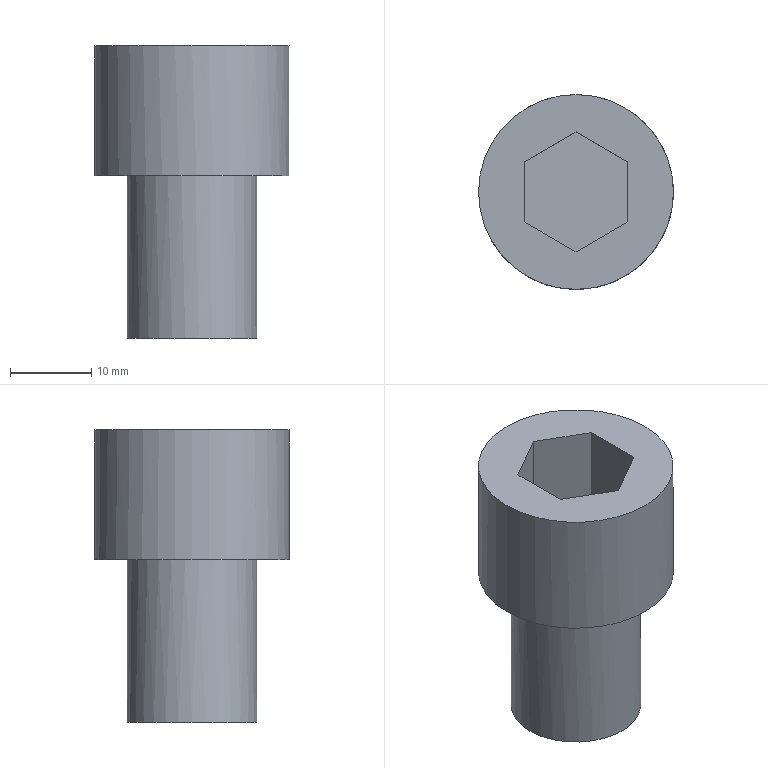Part | NX | features solid 2 | 1 solid | 12 faces | box 24 x 24 x 36 mm | volume 9897 mm3 | plane 10 | cylinder 2 | commonest cylinder face diameters 16 x1 24 x1
STEP:
#1=CARTESIAN_POINT('',(1036.4,273.695,-259.));
#2=VERTEX_POINT('',#1);
#3=CARTESIAN_POINT('',(1030.,277.39,-259.));
#4=VERTEX_POINT('',#3);
#5=CARTESIAN_POINT('',(1033.2,275.543,-259.));
#6=DIRECTION('',(-0.866,0.5,0.));
#7=VECTOR('',#6,1000.);
#8=LINE('',#5,#7);
#9=EDGE_CURVE('',#2,#4,#8,.T.);
#10=ORIENTED_EDGE('',*,*,#9,.F.);
#11=CARTESIAN_POINT('',(1036.4,266.305,-259.));
#12=VERTEX_POINT('',#11);
#13=CARTESIAN_POINT('',(1036.4,270.,-259.));
#14=DIRECTION('',(0.,1.,0.));
#15=VECTOR('',#14,1000.);
#16=LINE('',#13,#15);
#17=EDGE_CURVE('',#12,#2,#16,.T.);
#18=ORIENTED_EDGE('',*,*,#17,.F.);
#19=CARTESIAN_POINT('',(1030.,262.61,-259.));
#20=VERTEX_POINT('',#19);
#21=CARTESIAN_POINT('',(1033.2,264.457,-259.));
#22=DIRECTION('',(0.866,0.5,0.));
#23=VECTOR('',#22,1000.);
#24=LINE('',#21,#23);
#25=EDGE_CURVE('',#20,#12,#24,.T.);
#26=ORIENTED_EDGE('',*,*,#25,.F.);
#27=CARTESIAN_POINT('',(1023.6,266.305,-259.));
#28=VERTEX_POINT('',#27);
#29=CARTESIAN_POINT('',(1026.8,264.457,-259.));
#30=DIRECTION('',(0.866,-0.5,0.));
#31=VECTOR('',#30,1000.);
#32=LINE('',#29,#31);
#33=EDGE_CURVE('',#28,#20,#32,.T.);
#34=ORIENTED_EDGE('',*,*,#33,.F.);
#35=CARTESIAN_POINT('',(1023.6,273.695,-259.));
#36=VERTEX_POINT('',#35);
#37=CARTESIAN_POINT('',(1023.6,270.,-259.));
#38=DIRECTION('',(0.,-1.,0.));
#39=VECTOR('',#38,1000.);
#40=LINE('',#37,#39);
#41=EDGE_CURVE('',#36,#28,#40,.T.);
#42=ORIENTED_EDGE('',*,*,#41,.F.);
#43=CARTESIAN_POINT('',(1026.8,275.543,-259.));
#44=DIRECTION('',(-0.866,-0.5,0.));
#45=VECTOR('',#44,1000.);
#46=LINE('',#43,#45);
#47=EDGE_CURVE('',#4,#36,#46,.T.);
#48=ORIENTED_EDGE('',*,*,#47,.F.);
#49=EDGE_LOOP('',(#10,#18,#26,#34,#42,#48));
#50=FACE_BOUND('',#49,.T.);
#51=CARTESIAN_POINT('',(1042.,270.,-259.));
#52=VERTEX_POINT('',#51);
#53=CARTESIAN_POINT('',(1030.,270.,-259.));
#54=DIRECTION('',(0.,0.,-1.));
#55=DIRECTION('',(1.,0.,0.));
#56=AXIS2_PLACEMENT_3D('',#53,#54,#55);
#57=CIRCLE('',#56,12.);
#58=EDGE_CURVE('',#52,#52,#57,.T.);
#59=ORIENTED_EDGE('',*,*,#58,.F.);
#60=EDGE_LOOP('',(#59));
#61=FACE_BOUND('',#60,.T.);
#62=CARTESIAN_POINT('',(1030.,270.,-259.));
#63=DIRECTION('',(0.,0.,1.));
#64=DIRECTION('',(-1.,0.,0.));
#65=AXIS2_PLACEMENT_3D('',#62,#63,#64);
#66=PLANE('',#65);
#67=ADVANCED_FACE('',(#50,#61),#66,.T.);
#68=CARTESIAN_POINT('',(1038.,270.,-275.));
#69=VERTEX_POINT('',#68);
#70=CARTESIAN_POINT('',(1030.,270.,-275.));
#71=DIRECTION('',(0.,0.,-1.));
#72=DIRECTION('',(1.,0.,0.));
#73=AXIS2_PLACEMENT_3D('',#70,#71,#72);
#74=CIRCLE('',#73,8.);
#75=EDGE_CURVE('',#69,#69,#74,.T.);
#76=ORIENTED_EDGE('',*,*,#75,.F.);
#77=EDGE_LOOP('',(#76));
#78=FACE_BOUND('',#77,.T.);
#79=CARTESIAN_POINT('',(1018.,270.,-275.));
#80=VERTEX_POINT('',#79);
#81=CARTESIAN_POINT('',(1030.,270.,-275.));
#82=DIRECTION('',(0.,0.,1.));
#83=DIRECTION('',(-1.,0.,0.));
#84=AXIS2_PLACEMENT_3D('',#81,#82,#83);
#85=CIRCLE('',#84,12.);
#86=EDGE_CURVE('',#80,#80,#85,.T.);
#87=ORIENTED_EDGE('',*,*,#86,.F.);
#88=EDGE_LOOP('',(#87));
#89=FACE_BOUND('',#88,.T.);
#90=CARTESIAN_POINT('',(1030.,270.,-275.));
#91=DIRECTION('',(0.,0.,-1.));
#92=DIRECTION('',(1.,0.,0.));
#93=AXIS2_PLACEMENT_3D('',#90,#91,#92);
#94=PLANE('',#93);
#95=ADVANCED_FACE('',(#78,#89),#94,.T.);
#96=ORIENTED_EDGE('',*,*,#58,.T.);
#97=EDGE_LOOP('',(#96));
#98=FACE_BOUND('',#97,.T.);
#99=ORIENTED_EDGE('',*,*,#86,.T.);
#100=EDGE_LOOP('',(#99));
#101=FACE_BOUND('',#100,.T.);
#102=CARTESIAN_POINT('',(1030.,270.,-275.));
#103=DIRECTION('',(0.,0.,1.));
#104=DIRECTION('',(-1.,0.,0.));
#105=AXIS2_PLACEMENT_3D('',#102,#103,#104);
#106=CYLINDRICAL_SURFACE('',#105,12.);
#107=ADVANCED_FACE('',(#98,#101),#106,.T.);
#108=ORIENTED_EDGE('',*,*,#9,.T.);
#109=CARTESIAN_POINT('',(1030.,277.39,-268.6));
#110=VERTEX_POINT('',#109);
#111=CARTESIAN_POINT('',(1030.,277.39,-268.6));
#112=DIRECTION('',(0.,0.,1.));
#113=VECTOR('',#112,1000.);
#114=LINE('',#111,#113);
#115=EDGE_CURVE('',#110,#4,#114,.T.);
#116=ORIENTED_EDGE('',*,*,#115,.F.);
#117=CARTESIAN_POINT('',(1036.4,273.695,-268.6));
#118=VERTEX_POINT('',#117);
#119=CARTESIAN_POINT('',(1036.4,273.695,-268.6));
#120=DIRECTION('',(-0.866,0.5,0.));
#121=VECTOR('',#120,1000.);
#122=LINE('',#119,#121);
#123=EDGE_CURVE('',#118,#110,#122,.T.);
#124=ORIENTED_EDGE('',*,*,#123,.F.);
#125=CARTESIAN_POINT('',(1036.4,273.695,-268.6));
#126=DIRECTION('',(0.,0.,1.));
#127=VECTOR('',#126,1000.);
#128=LINE('',#125,#127);
#129=EDGE_CURVE('',#118,#2,#128,.T.);
#130=ORIENTED_EDGE('',*,*,#129,.T.);
#131=EDGE_LOOP('',(#108,#116,#124,#130));
#132=FACE_BOUND('',#131,.T.);
#133=CARTESIAN_POINT('',(1033.2,275.543,-260.6));
#134=DIRECTION('',(0.5,0.866,0.));
#135=DIRECTION('',(-0.866,0.5,0.));
#136=AXIS2_PLACEMENT_3D('',#133,#134,#135);
#137=PLANE('',#136);
#138=ADVANCED_FACE('',(#132),#137,.F.);
#139=ORIENTED_EDGE('',*,*,#17,.T.);
#140=ORIENTED_EDGE('',*,*,#129,.F.);
#141=CARTESIAN_POINT('',(1036.4,266.305,-268.6));
#142=VERTEX_POINT('',#141);
#143=CARTESIAN_POINT('',(1036.4,266.305,-268.6));
#144=DIRECTION('',(0.,1.,0.));
#145=VECTOR('',#144,1000.);
#146=LINE('',#143,#145);
#147=EDGE_CURVE('',#142,#118,#146,.T.);
#148=ORIENTED_EDGE('',*,*,#147,.F.);
#149=CARTESIAN_POINT('',(1036.4,266.305,-268.6));
#150=DIRECTION('',(0.,0.,1.));
#151=VECTOR('',#150,1000.);
#152=LINE('',#149,#151);
#153=EDGE_CURVE('',#142,#12,#152,.T.);
#154=ORIENTED_EDGE('',*,*,#153,.T.);
#155=EDGE_LOOP('',(#139,#140,#148,#154));
#156=FACE_BOUND('',#155,.T.);
#157=CARTESIAN_POINT('',(1036.4,270.,-260.6));
#158=DIRECTION('',(1.,0.,0.));
#159=DIRECTION('',(0.,0.,1.));
#160=AXIS2_PLACEMENT_3D('',#157,#158,#159);
#161=PLANE('',#160);
#162=ADVANCED_FACE('',(#156),#161,.F.);
#163=ORIENTED_EDGE('',*,*,#25,.T.);
#164=ORIENTED_EDGE('',*,*,#153,.F.);
#165=CARTESIAN_POINT('',(1030.,262.61,-268.6));
#166=VERTEX_POINT('',#165);
#167=CARTESIAN_POINT('',(1030.,262.61,-268.6));
#168=DIRECTION('',(0.866,0.5,0.));
#169=VECTOR('',#168,1000.);
#170=LINE('',#167,#169);
#171=EDGE_CURVE('',#166,#142,#170,.T.);
#172=ORIENTED_EDGE('',*,*,#171,.F.);
#173=CARTESIAN_POINT('',(1030.,262.61,-268.6));
#174=DIRECTION('',(0.,0.,1.));
#175=VECTOR('',#174,1000.);
#176=LINE('',#173,#175);
#177=EDGE_CURVE('',#166,#20,#176,.T.);
#178=ORIENTED_EDGE('',*,*,#177,.T.);
#179=EDGE_LOOP('',(#163,#164,#172,#178));
#180=FACE_BOUND('',#179,.T.);
#181=CARTESIAN_POINT('',(1033.2,264.457,-260.6));
#182=DIRECTION('',(0.5,-0.866,0.));
#183=DIRECTION('',(0.866,0.5,0.));
#184=AXIS2_PLACEMENT_3D('',#181,#182,#183);
#185=PLANE('',#184);
#186=ADVANCED_FACE('',(#180),#185,.F.);
#187=ORIENTED_EDGE('',*,*,#33,.T.);
#188=ORIENTED_EDGE('',*,*,#177,.F.);
#189=CARTESIAN_POINT('',(1023.6,266.305,-268.6));
#190=VERTEX_POINT('',#189);
#191=CARTESIAN_POINT('',(1023.6,266.305,-268.6));
#192=DIRECTION('',(0.866,-0.5,0.));
#193=VECTOR('',#192,1000.);
#194=LINE('',#191,#193);
#195=EDGE_CURVE('',#190,#166,#194,.T.);
#196=ORIENTED_EDGE('',*,*,#195,.F.);
#197=CARTESIAN_POINT('',(1023.6,266.305,-268.6));
#198=DIRECTION('',(0.,0.,1.));
#199=VECTOR('',#198,1000.);
#200=LINE('',#197,#199);
#201=EDGE_CURVE('',#190,#28,#200,.T.);
#202=ORIENTED_EDGE('',*,*,#201,.T.);
#203=EDGE_LOOP('',(#187,#188,#196,#202));
#204=FACE_BOUND('',#203,.T.);
#205=CARTESIAN_POINT('',(1026.8,264.457,-260.6));
#206=DIRECTION('',(-0.5,-0.866,0.));
#207=DIRECTION('',(0.866,-0.5,0.));
#208=AXIS2_PLACEMENT_3D('',#205,#206,#207);
#209=PLANE('',#208);
#210=ADVANCED_FACE('',(#204),#209,.F.);
#211=ORIENTED_EDGE('',*,*,#41,.T.);
#212=ORIENTED_EDGE('',*,*,#201,.F.);
#213=CARTESIAN_POINT('',(1023.6,273.695,-268.6));
#214=VERTEX_POINT('',#213);
#215=CARTESIAN_POINT('',(1023.6,273.695,-268.6));
#216=DIRECTION('',(0.,-1.,0.));
#217=VECTOR('',#216,1000.);
#218=LINE('',#215,#217);
#219=EDGE_CURVE('',#214,#190,#218,.T.);
#220=ORIENTED_EDGE('',*,*,#219,.F.);
#221=CARTESIAN_POINT('',(1023.6,273.695,-268.6));
#222=DIRECTION('',(0.,0.,1.));
#223=VECTOR('',#222,1000.);
#224=LINE('',#221,#223);
#225=EDGE_CURVE('',#214,#36,#224,.T.);
#226=ORIENTED_EDGE('',*,*,#225,.T.);
#227=EDGE_LOOP('',(#211,#212,#220,#226));
#228=FACE_BOUND('',#227,.T.);
#229=CARTESIAN_POINT('',(1023.6,270.,-260.6));
#230=DIRECTION('',(-1.,0.,0.));
#231=DIRECTION('',(0.,0.,-1.));
#232=AXIS2_PLACEMENT_3D('',#229,#230,#231);
#233=PLANE('',#232);
#234=ADVANCED_FACE('',(#228),#233,.F.);
#235=ORIENTED_EDGE('',*,*,#47,.T.);
#236=ORIENTED_EDGE('',*,*,#225,.F.);
#237=CARTESIAN_POINT('',(1030.,277.39,-268.6));
#238=DIRECTION('',(-0.866,-0.5,0.));
#239=VECTOR('',#238,1000.);
#240=LINE('',#237,#239);
#241=EDGE_CURVE('',#110,#214,#240,.T.);
#242=ORIENTED_EDGE('',*,*,#241,.F.);
#243=ORIENTED_EDGE('',*,*,#115,.T.);
#244=EDGE_LOOP('',(#235,#236,#242,#243));
#245=FACE_BOUND('',#244,.T.);
#246=CARTESIAN_POINT('',(1026.8,275.543,-260.6));
#247=DIRECTION('',(-0.5,0.866,0.));
#248=DIRECTION('',(-0.866,-0.5,0.));
#249=AXIS2_PLACEMENT_3D('',#246,#247,#248);
#250=PLANE('',#249);
#251=ADVANCED_FACE('',(#245),#250,.F.);
#252=ORIENTED_EDGE('',*,*,#241,.T.);
#253=ORIENTED_EDGE('',*,*,#219,.T.);
#254=ORIENTED_EDGE('',*,*,#195,.T.);
#255=ORIENTED_EDGE('',*,*,#171,.T.);
#256=ORIENTED_EDGE('',*,*,#147,.T.);
#257=ORIENTED_EDGE('',*,*,#123,.T.);
#258=EDGE_LOOP('',(#252,#253,#254,#255,#256,#257));
#259=FACE_BOUND('',#258,.T.);
#260=CARTESIAN_POINT('',(1030.,270.,-268.6));
#261=DIRECTION('',(0.,0.,-1.));
#262=DIRECTION('',(1.,0.,0.));
#263=AXIS2_PLACEMENT_3D('',#260,#261,#262);
#264=PLANE('',#263);
#265=ADVANCED_FACE('',(#259),#264,.F.);
#266=CARTESIAN_POINT('',(1022.,270.,-295.));
#267=VERTEX_POINT('',#266);
#268=CARTESIAN_POINT('',(1030.,270.,-295.));
#269=DIRECTION('',(0.,0.,1.));
#270=DIRECTION('',(-1.,0.,0.));
#271=AXIS2_PLACEMENT_3D('',#268,#269,#270);
#272=CIRCLE('',#271,8.);
#273=EDGE_CURVE('',#267,#267,#272,.T.);
#274=ORIENTED_EDGE('',*,*,#273,.F.);
#275=EDGE_LOOP('',(#274));
#276=FACE_BOUND('',#275,.T.);
#277=CARTESIAN_POINT('',(1030.,270.,-295.));
#278=DIRECTION('',(0.,0.,-1.));
#279=DIRECTION('',(1.,0.,0.));
#280=AXIS2_PLACEMENT_3D('',#277,#278,#279);
#281=PLANE('',#280);
#282=ADVANCED_FACE('',(#276),#281,.T.);
#283=ORIENTED_EDGE('',*,*,#273,.T.);
#284=EDGE_LOOP('',(#283));
#285=FACE_BOUND('',#284,.T.);
#286=ORIENTED_EDGE('',*,*,#75,.T.);
#287=EDGE_LOOP('',(#286));
#288=FACE_BOUND('',#287,.T.);
#289=CARTESIAN_POINT('',(1030.,270.,-275.));
#290=DIRECTION('',(0.,0.,-1.));
#291=DIRECTION('',(1.,0.,0.));
#292=AXIS2_PLACEMENT_3D('',#289,#290,#291);
#293=CYLINDRICAL_SURFACE('',#292,8.);
#294=ADVANCED_FACE('',(#285,#288),#293,.T.);
#295=CLOSED_SHELL('',(#67,#95,#107,#138,#162,#186,#210,#234,#251,#265,#282,#294));
#296=MANIFOLD_SOLID_BREP('',#295);
#297=(LENGTH_UNIT()NAMED_UNIT(*)SI_UNIT(.MILLI.,.METRE.));
#298=UNCERTAINTY_MEASURE_WITH_UNIT(LENGTH_MEASURE(0.00001),#297,'','');
#299=(NAMED_UNIT(*)PLANE_ANGLE_UNIT()SI_UNIT($,.RADIAN.));
#300=(NAMED_UNIT(*)SI_UNIT($,.STERADIAN.)SOLID_ANGLE_UNIT());
#301=(GEOMETRIC_REPRESENTATION_CONTEXT(3)GLOBAL_UNCERTAINTY_ASSIGNED_CONTEXT((#298))GLOBAL_UNIT_ASSIGNED_CONTEXT((#297,#299,#300))REPRESENTATION_CONTEXT('',''));
#302=ADVANCED_BREP_SHAPE_REPRESENTATION('',(#296),#301);